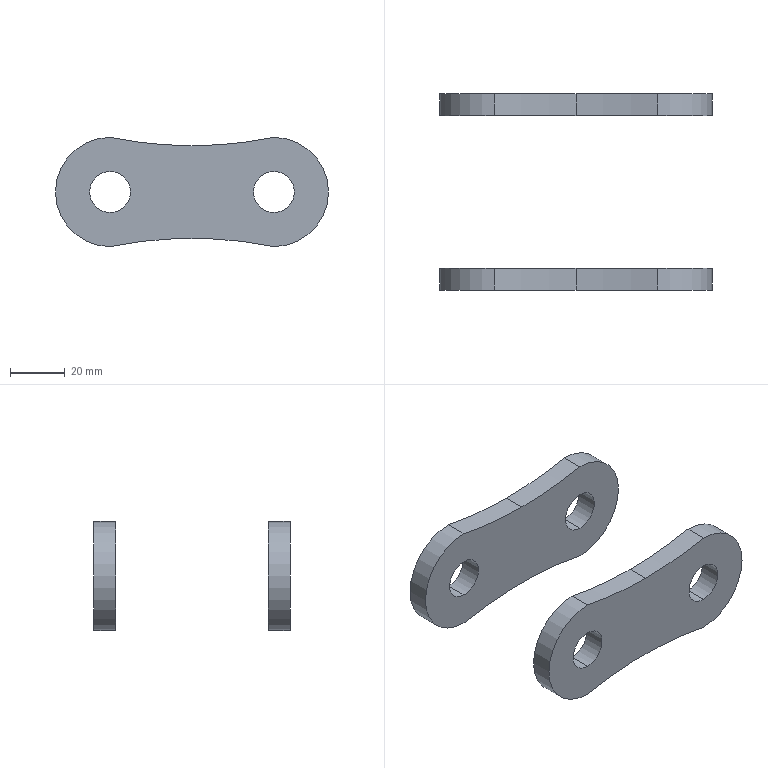Part | SolidWorks | features Extrusion 1, LPattern 1 | 2 solids | 22 faces | box 100 x 72 x 40 mm | volume 48964 mm3 | cylinder 18 | plane 4 | commonest cylinder face diameters 15 x8 300 x6 40 x4
STEP:
#1=CARTESIAN_POINT('',(60.,8.,-7.5));
#2=VERTEX_POINT('',#1);
#3=CARTESIAN_POINT('',(60.,8.,7.5));
#4=VERTEX_POINT('',#3);
#5=CARTESIAN_POINT('',(60.,8.,0.));
#6=DIRECTION('',(0.,1.,0.));
#7=DIRECTION('',(0.,0.,1.));
#8=AXIS2_PLACEMENT_3D('',#5,#6,#7);
#9=CIRCLE('',#8,7.5);
#10=EDGE_CURVE('',#2,#4,#9,.T.);
#11=ORIENTED_EDGE('',*,*,#10,.T.);
#12=CARTESIAN_POINT('',(60.,0.,7.5));
#13=VERTEX_POINT('',#12);
#14=CARTESIAN_POINT('',(60.,8.,7.5));
#15=DIRECTION('',(0.,-1.,0.));
#16=VECTOR('',#15,1000.);
#17=LINE('',#14,#16);
#18=EDGE_CURVE('',#4,#13,#17,.T.);
#19=ORIENTED_EDGE('',*,*,#18,.T.);
#20=CARTESIAN_POINT('',(60.,0.,-7.5));
#21=VERTEX_POINT('',#20);
#22=CARTESIAN_POINT('',(60.,0.,0.));
#23=DIRECTION('',(0.,1.,0.));
#24=DIRECTION('',(0.,0.,1.));
#25=AXIS2_PLACEMENT_3D('',#22,#23,#24);
#26=CIRCLE('',#25,7.5);
#27=EDGE_CURVE('',#21,#13,#26,.T.);
#28=ORIENTED_EDGE('',*,*,#27,.F.);
#29=CARTESIAN_POINT('',(60.,8.,-7.5));
#30=DIRECTION('',(0.,-1.,0.));
#31=VECTOR('',#30,1000.);
#32=LINE('',#29,#31);
#33=EDGE_CURVE('',#2,#21,#32,.T.);
#34=ORIENTED_EDGE('',*,*,#33,.F.);
#35=EDGE_LOOP('',(#11,#19,#28,#34));
#36=FACE_OUTER_BOUND('',#35,.T.);
#37=CARTESIAN_POINT('',(60.,8.,0.));
#38=DIRECTION('',(0.,-1.,0.));
#39=DIRECTION('',(0.,0.,-1.));
#40=AXIS2_PLACEMENT_3D('',#37,#38,#39);
#41=CYLINDRICAL_SURFACE('',#40,7.5);
#42=ADVANCED_FACE('',(#36),#41,.F.);
#43=CARTESIAN_POINT('',(0.,8.,-7.5));
#44=VERTEX_POINT('',#43);
#45=CARTESIAN_POINT('',(0.,8.,7.5));
#46=VERTEX_POINT('',#45);
#47=CARTESIAN_POINT('',(0.,8.,0.));
#48=DIRECTION('',(0.,1.,0.));
#49=DIRECTION('',(0.,0.,1.));
#50=AXIS2_PLACEMENT_3D('',#47,#48,#49);
#51=CIRCLE('',#50,7.5);
#52=EDGE_CURVE('',#44,#46,#51,.T.);
#53=ORIENTED_EDGE('',*,*,#52,.T.);
#54=CARTESIAN_POINT('',(0.,0.,7.5));
#55=VERTEX_POINT('',#54);
#56=CARTESIAN_POINT('',(0.,8.,7.5));
#57=DIRECTION('',(0.,-1.,0.));
#58=VECTOR('',#57,1000.);
#59=LINE('',#56,#58);
#60=EDGE_CURVE('',#46,#55,#59,.T.);
#61=ORIENTED_EDGE('',*,*,#60,.T.);
#62=CARTESIAN_POINT('',(0.,0.,-7.5));
#63=VERTEX_POINT('',#62);
#64=CARTESIAN_POINT('',(0.,0.,0.));
#65=DIRECTION('',(0.,1.,0.));
#66=DIRECTION('',(0.,0.,1.));
#67=AXIS2_PLACEMENT_3D('',#64,#65,#66);
#68=CIRCLE('',#67,7.5);
#69=EDGE_CURVE('',#63,#55,#68,.T.);
#70=ORIENTED_EDGE('',*,*,#69,.F.);
#71=CARTESIAN_POINT('',(0.,8.,-7.5));
#72=DIRECTION('',(0.,-1.,0.));
#73=VECTOR('',#72,1000.);
#74=LINE('',#71,#73);
#75=EDGE_CURVE('',#44,#63,#74,.T.);
#76=ORIENTED_EDGE('',*,*,#75,.F.);
#77=EDGE_LOOP('',(#53,#61,#70,#76));
#78=FACE_OUTER_BOUND('',#77,.T.);
#79=CARTESIAN_POINT('',(0.,8.,0.));
#80=DIRECTION('',(0.,-1.,0.));
#81=DIRECTION('',(0.,0.,-1.));
#82=AXIS2_PLACEMENT_3D('',#79,#80,#81);
#83=CYLINDRICAL_SURFACE('',#82,7.5);
#84=ADVANCED_FACE('',(#78),#83,.F.);
#85=CARTESIAN_POINT('',(30.,8.,16.969));
#86=VERTEX_POINT('',#85);
#87=CARTESIAN_POINT('',(60.,8.,20.));
#88=VERTEX_POINT('',#87);
#89=CARTESIAN_POINT('',(30.,8.,166.969));
#90=DIRECTION('',(0.,-1.,0.));
#91=DIRECTION('',(0.,0.,-1.));
#92=AXIS2_PLACEMENT_3D('',#89,#90,#91);
#93=CIRCLE('',#92,150.);
#94=EDGE_CURVE('',#86,#88,#93,.T.);
#95=ORIENTED_EDGE('',*,*,#94,.F.);
#96=CARTESIAN_POINT('',(30.,0.,16.969));
#97=VERTEX_POINT('',#96);
#98=CARTESIAN_POINT('',(30.,8.,16.969));
#99=DIRECTION('',(0.,-1.,0.));
#100=VECTOR('',#99,1000.);
#101=LINE('',#98,#100);
#102=EDGE_CURVE('',#86,#97,#101,.T.);
#103=ORIENTED_EDGE('',*,*,#102,.T.);
#104=CARTESIAN_POINT('',(60.,0.,20.));
#105=VERTEX_POINT('',#104);
#106=CARTESIAN_POINT('',(30.,0.,166.969));
#107=DIRECTION('',(0.,-1.,0.));
#108=DIRECTION('',(0.,0.,-1.));
#109=AXIS2_PLACEMENT_3D('',#106,#107,#108);
#110=CIRCLE('',#109,150.);
#111=EDGE_CURVE('',#97,#105,#110,.T.);
#112=ORIENTED_EDGE('',*,*,#111,.T.);
#113=CARTESIAN_POINT('',(60.,8.,20.));
#114=DIRECTION('',(0.,-1.,0.));
#115=VECTOR('',#114,1000.);
#116=LINE('',#113,#115);
#117=EDGE_CURVE('',#88,#105,#116,.T.);
#118=ORIENTED_EDGE('',*,*,#117,.F.);
#119=EDGE_LOOP('',(#95,#103,#112,#118));
#120=FACE_OUTER_BOUND('',#119,.T.);
#121=CARTESIAN_POINT('',(30.,8.,166.969));
#122=DIRECTION('',(0.,-1.,0.));
#123=DIRECTION('',(0.,0.,-1.));
#124=AXIS2_PLACEMENT_3D('',#121,#122,#123);
#125=CYLINDRICAL_SURFACE('',#124,150.);
#126=ADVANCED_FACE('',(#120),#125,.F.);
#127=ORIENTED_EDGE('',*,*,#52,.F.);
#128=CARTESIAN_POINT('',(0.,8.,0.));
#129=DIRECTION('',(0.,1.,0.));
#130=DIRECTION('',(0.,0.,1.));
#131=AXIS2_PLACEMENT_3D('',#128,#129,#130);
#132=CIRCLE('',#131,7.5);
#133=EDGE_CURVE('',#46,#44,#132,.T.);
#134=ORIENTED_EDGE('',*,*,#133,.F.);
#135=EDGE_LOOP('',(#127,#134));
#136=FACE_BOUND('',#135,.T.);
#137=CARTESIAN_POINT('',(60.,8.,-20.));
#138=VERTEX_POINT('',#137);
#139=CARTESIAN_POINT('',(0.,8.,-20.));
#140=VERTEX_POINT('',#139);
#141=CARTESIAN_POINT('',(30.,8.,-166.969));
#142=DIRECTION('',(0.,-1.,0.));
#143=DIRECTION('',(0.,0.,1.));
#144=AXIS2_PLACEMENT_3D('',#141,#142,#143);
#145=CIRCLE('',#144,150.);
#146=EDGE_CURVE('',#138,#140,#145,.T.);
#147=ORIENTED_EDGE('',*,*,#146,.T.);
#148=CARTESIAN_POINT('',(0.,8.,20.));
#149=VERTEX_POINT('',#148);
#150=CARTESIAN_POINT('',(0.,8.,0.));
#151=DIRECTION('',(0.,1.,0.));
#152=DIRECTION('',(0.,0.,1.));
#153=AXIS2_PLACEMENT_3D('',#150,#151,#152);
#154=CIRCLE('',#153,20.);
#155=EDGE_CURVE('',#140,#149,#154,.T.);
#156=ORIENTED_EDGE('',*,*,#155,.T.);
#157=CARTESIAN_POINT('',(30.,8.,166.969));
#158=DIRECTION('',(0.,-1.,0.));
#159=DIRECTION('',(0.,0.,-1.));
#160=AXIS2_PLACEMENT_3D('',#157,#158,#159);
#161=CIRCLE('',#160,150.);
#162=EDGE_CURVE('',#149,#86,#161,.T.);
#163=ORIENTED_EDGE('',*,*,#162,.T.);
#164=ORIENTED_EDGE('',*,*,#94,.T.);
#165=CARTESIAN_POINT('',(60.,8.,0.));
#166=DIRECTION('',(0.,1.,0.));
#167=DIRECTION('',(0.,0.,1.));
#168=AXIS2_PLACEMENT_3D('',#165,#166,#167);
#169=CIRCLE('',#168,20.);
#170=EDGE_CURVE('',#88,#138,#169,.T.);
#171=ORIENTED_EDGE('',*,*,#170,.T.);
#172=EDGE_LOOP('',(#147,#156,#163,#164,#171));
#173=FACE_OUTER_BOUND('',#172,.T.);
#174=ORIENTED_EDGE('',*,*,#10,.F.);
#175=CARTESIAN_POINT('',(60.,8.,0.));
#176=DIRECTION('',(0.,1.,0.));
#177=DIRECTION('',(0.,0.,1.));
#178=AXIS2_PLACEMENT_3D('',#175,#176,#177);
#179=CIRCLE('',#178,7.5);
#180=EDGE_CURVE('',#4,#2,#179,.T.);
#181=ORIENTED_EDGE('',*,*,#180,.F.);
#182=EDGE_LOOP('',(#174,#181));
#183=FACE_BOUND('',#182,.T.);
#184=CARTESIAN_POINT('',(45.,8.,-83.485));
#185=DIRECTION('',(0.,1.,0.));
#186=DIRECTION('',(0.,0.,1.));
#187=AXIS2_PLACEMENT_3D('',#184,#185,#186);
#188=PLANE('',#187);
#189=ADVANCED_FACE('',(#136,#173,#183),#188,.T.);
#190=CARTESIAN_POINT('',(60.,0.,-20.));
#191=VERTEX_POINT('',#190);
#192=CARTESIAN_POINT('',(0.,0.,-20.));
#193=VERTEX_POINT('',#192);
#194=CARTESIAN_POINT('',(30.,0.,-166.969));
#195=DIRECTION('',(0.,-1.,0.));
#196=DIRECTION('',(0.,0.,1.));
#197=AXIS2_PLACEMENT_3D('',#194,#195,#196);
#198=CIRCLE('',#197,150.);
#199=EDGE_CURVE('',#191,#193,#198,.T.);
#200=ORIENTED_EDGE('',*,*,#199,.F.);
#201=CARTESIAN_POINT('',(60.,0.,0.));
#202=DIRECTION('',(0.,1.,0.));
#203=DIRECTION('',(0.,0.,1.));
#204=AXIS2_PLACEMENT_3D('',#201,#202,#203);
#205=CIRCLE('',#204,20.);
#206=EDGE_CURVE('',#105,#191,#205,.T.);
#207=ORIENTED_EDGE('',*,*,#206,.F.);
#208=ORIENTED_EDGE('',*,*,#111,.F.);
#209=CARTESIAN_POINT('',(0.,0.,20.));
#210=VERTEX_POINT('',#209);
#211=CARTESIAN_POINT('',(30.,0.,166.969));
#212=DIRECTION('',(0.,-1.,0.));
#213=DIRECTION('',(0.,0.,-1.));
#214=AXIS2_PLACEMENT_3D('',#211,#212,#213);
#215=CIRCLE('',#214,150.);
#216=EDGE_CURVE('',#210,#97,#215,.T.);
#217=ORIENTED_EDGE('',*,*,#216,.F.);
#218=CARTESIAN_POINT('',(0.,0.,0.));
#219=DIRECTION('',(0.,1.,0.));
#220=DIRECTION('',(0.,0.,1.));
#221=AXIS2_PLACEMENT_3D('',#218,#219,#220);
#222=CIRCLE('',#221,20.);
#223=EDGE_CURVE('',#193,#210,#222,.T.);
#224=ORIENTED_EDGE('',*,*,#223,.F.);
#225=EDGE_LOOP('',(#200,#207,#208,#217,#224));
#226=FACE_OUTER_BOUND('',#225,.T.);
#227=ORIENTED_EDGE('',*,*,#69,.T.);
#228=CARTESIAN_POINT('',(0.,0.,0.));
#229=DIRECTION('',(0.,1.,0.));
#230=DIRECTION('',(0.,0.,1.));
#231=AXIS2_PLACEMENT_3D('',#228,#229,#230);
#232=CIRCLE('',#231,7.5);
#233=EDGE_CURVE('',#55,#63,#232,.T.);
#234=ORIENTED_EDGE('',*,*,#233,.T.);
#235=EDGE_LOOP('',(#227,#234));
#236=FACE_BOUND('',#235,.T.);
#237=ORIENTED_EDGE('',*,*,#27,.T.);
#238=CARTESIAN_POINT('',(60.,0.,0.));
#239=DIRECTION('',(0.,1.,0.));
#240=DIRECTION('',(0.,0.,1.));
#241=AXIS2_PLACEMENT_3D('',#238,#239,#240);
#242=CIRCLE('',#241,7.5);
#243=EDGE_CURVE('',#13,#21,#242,.T.);
#244=ORIENTED_EDGE('',*,*,#243,.T.);
#245=EDGE_LOOP('',(#237,#244));
#246=FACE_BOUND('',#245,.T.);
#247=CARTESIAN_POINT('',(45.,0.,-83.485));
#248=DIRECTION('',(0.,1.,0.));
#249=DIRECTION('',(0.,0.,1.));
#250=AXIS2_PLACEMENT_3D('',#247,#248,#249);
#251=PLANE('',#250);
#252=ADVANCED_FACE('',(#226,#236,#246),#251,.F.);
#253=ORIENTED_EDGE('',*,*,#199,.T.);
#254=CARTESIAN_POINT('',(0.,8.,-20.));
#255=DIRECTION('',(0.,-1.,0.));
#256=VECTOR('',#255,1000.);
#257=LINE('',#254,#256);
#258=EDGE_CURVE('',#140,#193,#257,.T.);
#259=ORIENTED_EDGE('',*,*,#258,.F.);
#260=ORIENTED_EDGE('',*,*,#146,.F.);
#261=CARTESIAN_POINT('',(60.,8.,-20.));
#262=DIRECTION('',(0.,-1.,0.));
#263=VECTOR('',#262,1000.);
#264=LINE('',#261,#263);
#265=EDGE_CURVE('',#138,#191,#264,.T.);
#266=ORIENTED_EDGE('',*,*,#265,.T.);
#267=EDGE_LOOP('',(#253,#259,#260,#266));
#268=FACE_OUTER_BOUND('',#267,.T.);
#269=CARTESIAN_POINT('',(30.,8.,-166.969));
#270=DIRECTION('',(0.,-1.,0.));
#271=DIRECTION('',(0.,0.,-1.));
#272=AXIS2_PLACEMENT_3D('',#269,#270,#271);
#273=CYLINDRICAL_SURFACE('',#272,150.);
#274=ADVANCED_FACE('',(#268),#273,.F.);
#275=ORIENTED_EDGE('',*,*,#223,.T.);
#276=CARTESIAN_POINT('',(0.,8.,20.));
#277=DIRECTION('',(0.,-1.,0.));
#278=VECTOR('',#277,1000.);
#279=LINE('',#276,#278);
#280=EDGE_CURVE('',#149,#210,#279,.T.);
#281=ORIENTED_EDGE('',*,*,#280,.F.);
#282=ORIENTED_EDGE('',*,*,#155,.F.);
#283=ORIENTED_EDGE('',*,*,#258,.T.);
#284=EDGE_LOOP('',(#275,#281,#282,#283));
#285=FACE_OUTER_BOUND('',#284,.T.);
#286=CARTESIAN_POINT('',(0.,8.,0.));
#287=DIRECTION('',(0.,-1.,0.));
#288=DIRECTION('',(0.,0.,-1.));
#289=AXIS2_PLACEMENT_3D('',#286,#287,#288);
#290=CYLINDRICAL_SURFACE('',#289,20.);
#291=ADVANCED_FACE('',(#285),#290,.T.);
#292=ORIENTED_EDGE('',*,*,#102,.F.);
#293=ORIENTED_EDGE('',*,*,#162,.F.);
#294=ORIENTED_EDGE('',*,*,#280,.T.);
#295=ORIENTED_EDGE('',*,*,#216,.T.);
#296=EDGE_LOOP('',(#292,#293,#294,#295));
#297=FACE_OUTER_BOUND('',#296,.T.);
#298=CARTESIAN_POINT('',(30.,8.,166.969));
#299=DIRECTION('',(0.,-1.,0.));
#300=DIRECTION('',(0.,0.,-1.));
#301=AXIS2_PLACEMENT_3D('',#298,#299,#300);
#302=CYLINDRICAL_SURFACE('',#301,150.);
#303=ADVANCED_FACE('',(#297),#302,.F.);
#304=ORIENTED_EDGE('',*,*,#206,.T.);
#305=ORIENTED_EDGE('',*,*,#265,.F.);
#306=ORIENTED_EDGE('',*,*,#170,.F.);
#307=ORIENTED_EDGE('',*,*,#117,.T.);
#308=EDGE_LOOP('',(#304,#305,#306,#307));
#309=FACE_OUTER_BOUND('',#308,.T.);
#310=CARTESIAN_POINT('',(60.,8.,0.));
#311=DIRECTION('',(0.,-1.,0.));
#312=DIRECTION('',(0.,0.,-1.));
#313=AXIS2_PLACEMENT_3D('',#310,#311,#312);
#314=CYLINDRICAL_SURFACE('',#313,20.);
#315=ADVANCED_FACE('',(#309),#314,.T.);
#316=ORIENTED_EDGE('',*,*,#60,.F.);
#317=ORIENTED_EDGE('',*,*,#133,.T.);
#318=ORIENTED_EDGE('',*,*,#75,.T.);
#319=ORIENTED_EDGE('',*,*,#233,.F.);
#320=EDGE_LOOP('',(#316,#317,#318,#319));
#321=FACE_OUTER_BOUND('',#320,.T.);
#322=CARTESIAN_POINT('',(0.,8.,0.));
#323=DIRECTION('',(0.,-1.,0.));
#324=DIRECTION('',(0.,0.,-1.));
#325=AXIS2_PLACEMENT_3D('',#322,#323,#324);
#326=CYLINDRICAL_SURFACE('',#325,7.5);
#327=ADVANCED_FACE('',(#321),#326,.F.);
#328=ORIENTED_EDGE('',*,*,#18,.F.);
#329=ORIENTED_EDGE('',*,*,#180,.T.);
#330=ORIENTED_EDGE('',*,*,#33,.T.);
#331=ORIENTED_EDGE('',*,*,#243,.F.);
#332=EDGE_LOOP('',(#328,#329,#330,#331));
#333=FACE_OUTER_BOUND('',#332,.T.);
#334=CARTESIAN_POINT('',(60.,8.,0.));
#335=DIRECTION('',(0.,-1.,0.));
#336=DIRECTION('',(0.,0.,-1.));
#337=AXIS2_PLACEMENT_3D('',#334,#335,#336);
#338=CYLINDRICAL_SURFACE('',#337,7.5);
#339=ADVANCED_FACE('',(#333),#338,.F.);
#340=CLOSED_SHELL('',(#42,#84,#126,#189,#252,#274,#291,#303,#315,#327,#339));
#341=MANIFOLD_SOLID_BREP('',#340);
#342=CARTESIAN_POINT('',(60.,72.,-7.5));
#343=VERTEX_POINT('',#342);
#344=CARTESIAN_POINT('',(60.,72.,7.5));
#345=VERTEX_POINT('',#344);
#346=CARTESIAN_POINT('',(60.,72.,0.));
#347=DIRECTION('',(0.,1.,0.));
#348=DIRECTION('',(0.,0.,1.));
#349=AXIS2_PLACEMENT_3D('',#346,#347,#348);
#350=CIRCLE('',#349,7.5);
#351=EDGE_CURVE('',#343,#345,#350,.T.);
#352=ORIENTED_EDGE('',*,*,#351,.T.);
#353=CARTESIAN_POINT('',(60.,64.,7.5));
#354=VERTEX_POINT('',#353);
#355=CARTESIAN_POINT('',(60.,72.,7.5));
#356=DIRECTION('',(0.,-1.,0.));
#357=VECTOR('',#356,1000.);
#358=LINE('',#355,#357);
#359=EDGE_CURVE('',#345,#354,#358,.T.);
#360=ORIENTED_EDGE('',*,*,#359,.T.);
#361=CARTESIAN_POINT('',(60.,64.,-7.5));
#362=VERTEX_POINT('',#361);
#363=CARTESIAN_POINT('',(60.,64.,0.));
#364=DIRECTION('',(0.,1.,0.));
#365=DIRECTION('',(0.,0.,1.));
#366=AXIS2_PLACEMENT_3D('',#363,#364,#365);
#367=CIRCLE('',#366,7.5);
#368=EDGE_CURVE('',#362,#354,#367,.T.);
#369=ORIENTED_EDGE('',*,*,#368,.F.);
#370=CARTESIAN_POINT('',(60.,72.,-7.5));
#371=DIRECTION('',(0.,-1.,0.));
#372=VECTOR('',#371,1000.);
#373=LINE('',#370,#372);
#374=EDGE_CURVE('',#343,#362,#373,.T.);
#375=ORIENTED_EDGE('',*,*,#374,.F.);
#376=EDGE_LOOP('',(#352,#360,#369,#375));
#377=FACE_OUTER_BOUND('',#376,.T.);
#378=CARTESIAN_POINT('',(60.,72.,0.));
#379=DIRECTION('',(0.,-1.,0.));
#380=DIRECTION('',(0.,0.,-1.));
#381=AXIS2_PLACEMENT_3D('',#378,#379,#380);
#382=CYLINDRICAL_SURFACE('',#381,7.5);
#383=ADVANCED_FACE('',(#377),#382,.F.);
#384=CARTESIAN_POINT('',(0.,72.,-7.5));
#385=VERTEX_POINT('',#384);
#386=CARTESIAN_POINT('',(0.,72.,7.5));
#387=VERTEX_POINT('',#386);
#388=CARTESIAN_POINT('',(0.,72.,0.));
#389=DIRECTION('',(0.,1.,0.));
#390=DIRECTION('',(0.,0.,1.));
#391=AXIS2_PLACEMENT_3D('',#388,#389,#390);
#392=CIRCLE('',#391,7.5);
#393=EDGE_CURVE('',#385,#387,#392,.T.);
#394=ORIENTED_EDGE('',*,*,#393,.T.);
#395=CARTESIAN_POINT('',(0.,64.,7.5));
#396=VERTEX_POINT('',#395);
#397=CARTESIAN_POINT('',(0.,72.,7.5));
#398=DIRECTION('',(0.,-1.,0.));
#399=VECTOR('',#398,1000.);
#400=LINE('',#397,#399);
#401=EDGE_CURVE('',#387,#396,#400,.T.);
#402=ORIENTED_EDGE('',*,*,#401,.T.);
#403=CARTESIAN_POINT('',(0.,64.,-7.5));
#404=VERTEX_POINT('',#403);
#405=CARTESIAN_POINT('',(0.,64.,0.));
#406=DIRECTION('',(0.,1.,0.));
#407=DIRECTION('',(0.,0.,1.));
#408=AXIS2_PLACEMENT_3D('',#405,#406,#407);
#409=CIRCLE('',#408,7.5);
#410=EDGE_CURVE('',#404,#396,#409,.T.);
#411=ORIENTED_EDGE('',*,*,#410,.F.);
#412=CARTESIAN_POINT('',(0.,72.,-7.5));
#413=DIRECTION('',(0.,-1.,0.));
#414=VECTOR('',#413,1000.);
#415=LINE('',#412,#414);
#416=EDGE_CURVE('',#385,#404,#415,.T.);
#417=ORIENTED_EDGE('',*,*,#416,.F.);
#418=EDGE_LOOP('',(#394,#402,#411,#417));
#419=FACE_OUTER_BOUND('',#418,.T.);
#420=CARTESIAN_POINT('',(0.,72.,0.));
#421=DIRECTION('',(0.,-1.,0.));
#422=DIRECTION('',(0.,0.,-1.));
#423=AXIS2_PLACEMENT_3D('',#420,#421,#422);
#424=CYLINDRICAL_SURFACE('',#423,7.5);
#425=ADVANCED_FACE('',(#419),#424,.F.);
#426=CARTESIAN_POINT('',(30.,72.,16.969));
#427=VERTEX_POINT('',#426);
#428=CARTESIAN_POINT('',(60.,72.,20.));
#429=VERTEX_POINT('',#428);
#430=CARTESIAN_POINT('',(30.,72.,166.969));
#431=DIRECTION('',(0.,-1.,0.));
#432=DIRECTION('',(0.,0.,-1.));
#433=AXIS2_PLACEMENT_3D('',#430,#431,#432);
#434=CIRCLE('',#433,150.);
#435=EDGE_CURVE('',#427,#429,#434,.T.);
#436=ORIENTED_EDGE('',*,*,#435,.F.);
#437=CARTESIAN_POINT('',(30.,64.,16.969));
#438=VERTEX_POINT('',#437);
#439=CARTESIAN_POINT('',(30.,72.,16.969));
#440=DIRECTION('',(0.,-1.,0.));
#441=VECTOR('',#440,1000.);
#442=LINE('',#439,#441);
#443=EDGE_CURVE('',#427,#438,#442,.T.);
#444=ORIENTED_EDGE('',*,*,#443,.T.);
#445=CARTESIAN_POINT('',(60.,64.,20.));
#446=VERTEX_POINT('',#445);
#447=CARTESIAN_POINT('',(30.,64.,166.969));
#448=DIRECTION('',(0.,-1.,0.));
#449=DIRECTION('',(0.,0.,-1.));
#450=AXIS2_PLACEMENT_3D('',#447,#448,#449);
#451=CIRCLE('',#450,150.);
#452=EDGE_CURVE('',#438,#446,#451,.T.);
#453=ORIENTED_EDGE('',*,*,#452,.T.);
#454=CARTESIAN_POINT('',(60.,72.,20.));
#455=DIRECTION('',(0.,-1.,0.));
#456=VECTOR('',#455,1000.);
#457=LINE('',#454,#456);
#458=EDGE_CURVE('',#429,#446,#457,.T.);
#459=ORIENTED_EDGE('',*,*,#458,.F.);
#460=EDGE_LOOP('',(#436,#444,#453,#459));
#461=FACE_OUTER_BOUND('',#460,.T.);
#462=CARTESIAN_POINT('',(30.,72.,166.969));
#463=DIRECTION('',(0.,-1.,0.));
#464=DIRECTION('',(0.,0.,-1.));
#465=AXIS2_PLACEMENT_3D('',#462,#463,#464);
#466=CYLINDRICAL_SURFACE('',#465,150.);
#467=ADVANCED_FACE('',(#461),#466,.F.);
#468=ORIENTED_EDGE('',*,*,#393,.F.);
#469=CARTESIAN_POINT('',(0.,72.,0.));
#470=DIRECTION('',(0.,1.,0.));
#471=DIRECTION('',(0.,0.,1.));
#472=AXIS2_PLACEMENT_3D('',#469,#470,#471);
#473=CIRCLE('',#472,7.5);
#474=EDGE_CURVE('',#387,#385,#473,.T.);
#475=ORIENTED_EDGE('',*,*,#474,.F.);
#476=EDGE_LOOP('',(#468,#475));
#477=FACE_BOUND('',#476,.T.);
#478=CARTESIAN_POINT('',(60.,72.,-20.));
#479=VERTEX_POINT('',#478);
#480=CARTESIAN_POINT('',(0.,72.,-20.));
#481=VERTEX_POINT('',#480);
#482=CARTESIAN_POINT('',(30.,72.,-166.969));
#483=DIRECTION('',(0.,-1.,0.));
#484=DIRECTION('',(0.,0.,1.));
#485=AXIS2_PLACEMENT_3D('',#482,#483,#484);
#486=CIRCLE('',#485,150.);
#487=EDGE_CURVE('',#479,#481,#486,.T.);
#488=ORIENTED_EDGE('',*,*,#487,.T.);
#489=CARTESIAN_POINT('',(0.,72.,20.));
#490=VERTEX_POINT('',#489);
#491=CARTESIAN_POINT('',(0.,72.,0.));
#492=DIRECTION('',(0.,1.,0.));
#493=DIRECTION('',(0.,0.,1.));
#494=AXIS2_PLACEMENT_3D('',#491,#492,#493);
#495=CIRCLE('',#494,20.);
#496=EDGE_CURVE('',#481,#490,#495,.T.);
#497=ORIENTED_EDGE('',*,*,#496,.T.);
#498=CARTESIAN_POINT('',(30.,72.,166.969));
#499=DIRECTION('',(0.,-1.,0.));
#500=DIRECTION('',(0.,0.,-1.));
#501=AXIS2_PLACEMENT_3D('',#498,#499,#500);
#502=CIRCLE('',#501,150.);
#503=EDGE_CURVE('',#490,#427,#502,.T.);
#504=ORIENTED_EDGE('',*,*,#503,.T.);
#505=ORIENTED_EDGE('',*,*,#435,.T.);
#506=CARTESIAN_POINT('',(60.,72.,0.));
#507=DIRECTION('',(0.,1.,0.));
#508=DIRECTION('',(0.,0.,1.));
#509=AXIS2_PLACEMENT_3D('',#506,#507,#508);
#510=CIRCLE('',#509,20.);
#511=EDGE_CURVE('',#429,#479,#510,.T.);
#512=ORIENTED_EDGE('',*,*,#511,.T.);
#513=EDGE_LOOP('',(#488,#497,#504,#505,#512));
#514=FACE_OUTER_BOUND('',#513,.T.);
#515=ORIENTED_EDGE('',*,*,#351,.F.);
#516=CARTESIAN_POINT('',(60.,72.,0.));
#517=DIRECTION('',(0.,1.,0.));
#518=DIRECTION('',(0.,0.,1.));
#519=AXIS2_PLACEMENT_3D('',#516,#517,#518);
#520=CIRCLE('',#519,7.5);
#521=EDGE_CURVE('',#345,#343,#520,.T.);
#522=ORIENTED_EDGE('',*,*,#521,.F.);
#523=EDGE_LOOP('',(#515,#522));
#524=FACE_BOUND('',#523,.T.);
#525=CARTESIAN_POINT('',(45.,72.,-83.485));
#526=DIRECTION('',(0.,1.,0.));
#527=DIRECTION('',(0.,0.,1.));
#528=AXIS2_PLACEMENT_3D('',#525,#526,#527);
#529=PLANE('',#528);
#530=ADVANCED_FACE('',(#477,#514,#524),#529,.T.);
#531=CARTESIAN_POINT('',(60.,64.,-20.));
#532=VERTEX_POINT('',#531);
#533=CARTESIAN_POINT('',(0.,64.,-20.));
#534=VERTEX_POINT('',#533);
#535=CARTESIAN_POINT('',(30.,64.,-166.969));
#536=DIRECTION('',(0.,-1.,0.));
#537=DIRECTION('',(0.,0.,1.));
#538=AXIS2_PLACEMENT_3D('',#535,#536,#537);
#539=CIRCLE('',#538,150.);
#540=EDGE_CURVE('',#532,#534,#539,.T.);
#541=ORIENTED_EDGE('',*,*,#540,.F.);
#542=CARTESIAN_POINT('',(60.,64.,0.));
#543=DIRECTION('',(0.,1.,0.));
#544=DIRECTION('',(0.,0.,1.));
#545=AXIS2_PLACEMENT_3D('',#542,#543,#544);
#546=CIRCLE('',#545,20.);
#547=EDGE_CURVE('',#446,#532,#546,.T.);
#548=ORIENTED_EDGE('',*,*,#547,.F.);
#549=ORIENTED_EDGE('',*,*,#452,.F.);
#550=CARTESIAN_POINT('',(0.,64.,20.));
#551=VERTEX_POINT('',#550);
#552=CARTESIAN_POINT('',(30.,64.,166.969));
#553=DIRECTION('',(0.,-1.,0.));
#554=DIRECTION('',(0.,0.,-1.));
#555=AXIS2_PLACEMENT_3D('',#552,#553,#554);
#556=CIRCLE('',#555,150.);
#557=EDGE_CURVE('',#551,#438,#556,.T.);
#558=ORIENTED_EDGE('',*,*,#557,.F.);
#559=CARTESIAN_POINT('',(0.,64.,0.));
#560=DIRECTION('',(0.,1.,0.));
#561=DIRECTION('',(0.,0.,1.));
#562=AXIS2_PLACEMENT_3D('',#559,#560,#561);
#563=CIRCLE('',#562,20.);
#564=EDGE_CURVE('',#534,#551,#563,.T.);
#565=ORIENTED_EDGE('',*,*,#564,.F.);
#566=EDGE_LOOP('',(#541,#548,#549,#558,#565));
#567=FACE_OUTER_BOUND('',#566,.T.);
#568=ORIENTED_EDGE('',*,*,#410,.T.);
#569=CARTESIAN_POINT('',(0.,64.,0.));
#570=DIRECTION('',(0.,1.,0.));
#571=DIRECTION('',(0.,0.,1.));
#572=AXIS2_PLACEMENT_3D('',#569,#570,#571);
#573=CIRCLE('',#572,7.5);
#574=EDGE_CURVE('',#396,#404,#573,.T.);
#575=ORIENTED_EDGE('',*,*,#574,.T.);
#576=EDGE_LOOP('',(#568,#575));
#577=FACE_BOUND('',#576,.T.);
#578=ORIENTED_EDGE('',*,*,#368,.T.);
#579=CARTESIAN_POINT('',(60.,64.,0.));
#580=DIRECTION('',(0.,1.,0.));
#581=DIRECTION('',(0.,0.,1.));
#582=AXIS2_PLACEMENT_3D('',#579,#580,#581);
#583=CIRCLE('',#582,7.5);
#584=EDGE_CURVE('',#354,#362,#583,.T.);
#585=ORIENTED_EDGE('',*,*,#584,.T.);
#586=EDGE_LOOP('',(#578,#585));
#587=FACE_BOUND('',#586,.T.);
#588=CARTESIAN_POINT('',(45.,64.,-83.485));
#589=DIRECTION('',(0.,1.,0.));
#590=DIRECTION('',(0.,0.,1.));
#591=AXIS2_PLACEMENT_3D('',#588,#589,#590);
#592=PLANE('',#591);
#593=ADVANCED_FACE('',(#567,#577,#587),#592,.F.);
#594=ORIENTED_EDGE('',*,*,#540,.T.);
#595=CARTESIAN_POINT('',(0.,72.,-20.));
#596=DIRECTION('',(0.,-1.,0.));
#597=VECTOR('',#596,1000.);
#598=LINE('',#595,#597);
#599=EDGE_CURVE('',#481,#534,#598,.T.);
#600=ORIENTED_EDGE('',*,*,#599,.F.);
#601=ORIENTED_EDGE('',*,*,#487,.F.);
#602=CARTESIAN_POINT('',(60.,72.,-20.));
#603=DIRECTION('',(0.,-1.,0.));
#604=VECTOR('',#603,1000.);
#605=LINE('',#602,#604);
#606=EDGE_CURVE('',#479,#532,#605,.T.);
#607=ORIENTED_EDGE('',*,*,#606,.T.);
#608=EDGE_LOOP('',(#594,#600,#601,#607));
#609=FACE_OUTER_BOUND('',#608,.T.);
#610=CARTESIAN_POINT('',(30.,72.,-166.969));
#611=DIRECTION('',(0.,-1.,0.));
#612=DIRECTION('',(0.,0.,-1.));
#613=AXIS2_PLACEMENT_3D('',#610,#611,#612);
#614=CYLINDRICAL_SURFACE('',#613,150.);
#615=ADVANCED_FACE('',(#609),#614,.F.);
#616=ORIENTED_EDGE('',*,*,#564,.T.);
#617=CARTESIAN_POINT('',(0.,72.,20.));
#618=DIRECTION('',(0.,-1.,0.));
#619=VECTOR('',#618,1000.);
#620=LINE('',#617,#619);
#621=EDGE_CURVE('',#490,#551,#620,.T.);
#622=ORIENTED_EDGE('',*,*,#621,.F.);
#623=ORIENTED_EDGE('',*,*,#496,.F.);
#624=ORIENTED_EDGE('',*,*,#599,.T.);
#625=EDGE_LOOP('',(#616,#622,#623,#624));
#626=FACE_OUTER_BOUND('',#625,.T.);
#627=CARTESIAN_POINT('',(0.,72.,0.));
#628=DIRECTION('',(0.,-1.,0.));
#629=DIRECTION('',(0.,0.,-1.));
#630=AXIS2_PLACEMENT_3D('',#627,#628,#629);
#631=CYLINDRICAL_SURFACE('',#630,20.);
#632=ADVANCED_FACE('',(#626),#631,.T.);
#633=ORIENTED_EDGE('',*,*,#443,.F.);
#634=ORIENTED_EDGE('',*,*,#503,.F.);
#635=ORIENTED_EDGE('',*,*,#621,.T.);
#636=ORIENTED_EDGE('',*,*,#557,.T.);
#637=EDGE_LOOP('',(#633,#634,#635,#636));
#638=FACE_OUTER_BOUND('',#637,.T.);
#639=CARTESIAN_POINT('',(30.,72.,166.969));
#640=DIRECTION('',(0.,-1.,0.));
#641=DIRECTION('',(0.,0.,-1.));
#642=AXIS2_PLACEMENT_3D('',#639,#640,#641);
#643=CYLINDRICAL_SURFACE('',#642,150.);
#644=ADVANCED_FACE('',(#638),#643,.F.);
#645=ORIENTED_EDGE('',*,*,#547,.T.);
#646=ORIENTED_EDGE('',*,*,#606,.F.);
#647=ORIENTED_EDGE('',*,*,#511,.F.);
#648=ORIENTED_EDGE('',*,*,#458,.T.);
#649=EDGE_LOOP('',(#645,#646,#647,#648));
#650=FACE_OUTER_BOUND('',#649,.T.);
#651=CARTESIAN_POINT('',(60.,72.,0.));
#652=DIRECTION('',(0.,-1.,0.));
#653=DIRECTION('',(0.,0.,-1.));
#654=AXIS2_PLACEMENT_3D('',#651,#652,#653);
#655=CYLINDRICAL_SURFACE('',#654,20.);
#656=ADVANCED_FACE('',(#650),#655,.T.);
#657=ORIENTED_EDGE('',*,*,#401,.F.);
#658=ORIENTED_EDGE('',*,*,#474,.T.);
#659=ORIENTED_EDGE('',*,*,#416,.T.);
#660=ORIENTED_EDGE('',*,*,#574,.F.);
#661=EDGE_LOOP('',(#657,#658,#659,#660));
#662=FACE_OUTER_BOUND('',#661,.T.);
#663=CARTESIAN_POINT('',(0.,72.,0.));
#664=DIRECTION('',(0.,-1.,0.));
#665=DIRECTION('',(0.,0.,-1.));
#666=AXIS2_PLACEMENT_3D('',#663,#664,#665);
#667=CYLINDRICAL_SURFACE('',#666,7.5);
#668=ADVANCED_FACE('',(#662),#667,.F.);
#669=ORIENTED_EDGE('',*,*,#359,.F.);
#670=ORIENTED_EDGE('',*,*,#521,.T.);
#671=ORIENTED_EDGE('',*,*,#374,.T.);
#672=ORIENTED_EDGE('',*,*,#584,.F.);
#673=EDGE_LOOP('',(#669,#670,#671,#672));
#674=FACE_OUTER_BOUND('',#673,.T.);
#675=CARTESIAN_POINT('',(60.,72.,0.));
#676=DIRECTION('',(0.,-1.,0.));
#677=DIRECTION('',(0.,0.,-1.));
#678=AXIS2_PLACEMENT_3D('',#675,#676,#677);
#679=CYLINDRICAL_SURFACE('',#678,7.5);
#680=ADVANCED_FACE('',(#674),#679,.F.);
#681=CLOSED_SHELL('',(#383,#425,#467,#530,#593,#615,#632,#644,#656,#668,#680));
#682=MANIFOLD_SOLID_BREP('',#681);
#683=CARTESIAN_POINT('',(0.,0.,0.));
#684=DIRECTION('',(0.,0.,1.));
#685=DIRECTION('',(1.,0.,0.));
#686=AXIS2_PLACEMENT_3D('',#683,#684,#685);
#687=(LENGTH_UNIT()NAMED_UNIT(*)SI_UNIT(.MILLI.,.METRE.));
#688=UNCERTAINTY_MEASURE_WITH_UNIT(LENGTH_MEASURE(0.00001),#687,'','');
#689=(NAMED_UNIT(*)PLANE_ANGLE_UNIT()SI_UNIT($,.RADIAN.));
#690=(NAMED_UNIT(*)SI_UNIT($,.STERADIAN.)SOLID_ANGLE_UNIT());
#691=(GEOMETRIC_REPRESENTATION_CONTEXT(3)GLOBAL_UNCERTAINTY_ASSIGNED_CONTEXT((#688))GLOBAL_UNIT_ASSIGNED_CONTEXT((#687,#689,#690))REPRESENTATION_CONTEXT('',''));
#692=ADVANCED_BREP_SHAPE_REPRESENTATION('',(#341,#682,#686),#691);